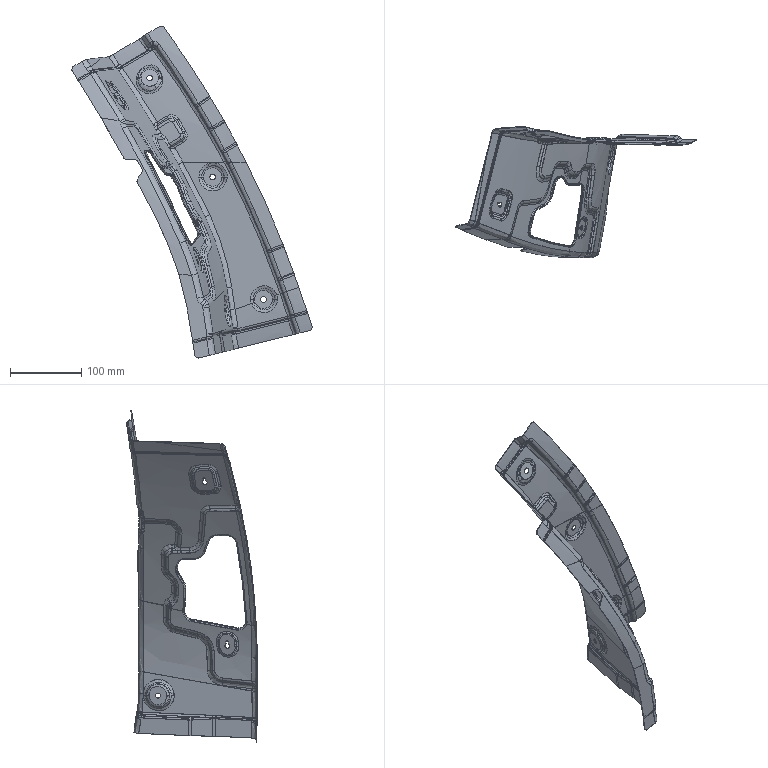Part | STEP file | FNA5401751 | 1 solid | 886 faces | box 337.448 x 183.804 x 466.44 mm | volume 116548 mm3 | spline 740 | cylinder 68 | plane 42 | other 20 | sphere 16 | commonest cylinder face diameters 8 x11 6 x5 10 x5 12 x5 2 x4 7 x4